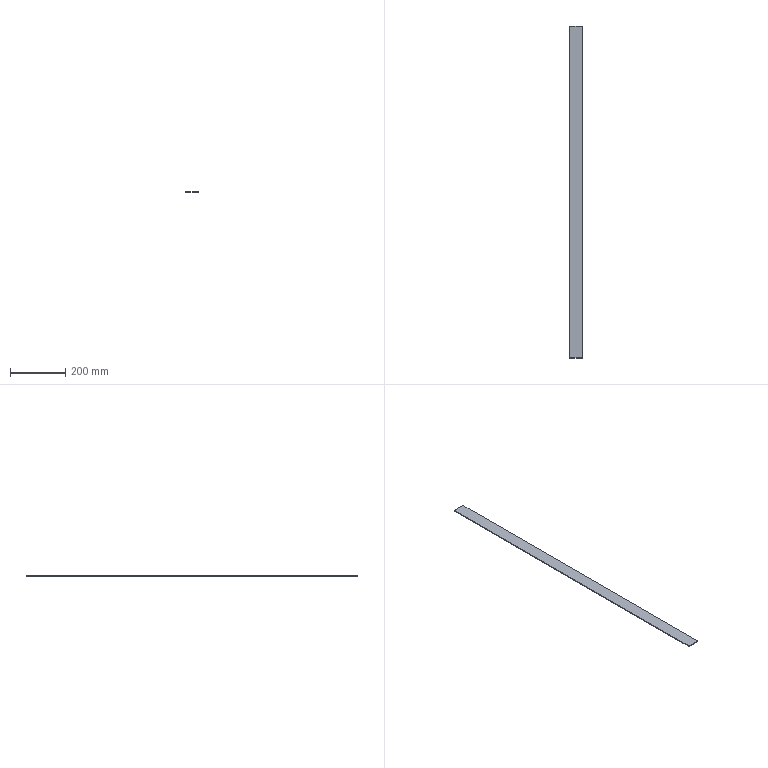Part | SolidWorks | features BaseBody 1 | 1 solid | 6 faces | box 44.635 x 1200 x 3 mm | volume 160685 mm3 | plane 6
STEP:
#1=CARTESIAN_POINT('',(171.506,600.,-1.5));
#2=VERTEX_POINT('',#1);
#3=CARTESIAN_POINT('',(171.506,-600.,-1.5));
#4=VERTEX_POINT('',#3);
#5=CARTESIAN_POINT('',(171.506,0.,-1.5));
#6=DIRECTION('',(0.,-1.,0.));
#7=VECTOR('',#6,1000.);
#8=LINE('',#5,#7);
#9=EDGE_CURVE('',#2,#4,#8,.T.);
#10=ORIENTED_EDGE('',*,*,#9,.T.);
#11=CARTESIAN_POINT('',(126.872,-600.,-1.5));
#12=VERTEX_POINT('',#11);
#13=CARTESIAN_POINT('',(149.189,-600.,-1.5));
#14=DIRECTION('',(-1.,0.,0.));
#15=VECTOR('',#14,1000.);
#16=LINE('',#13,#15);
#17=EDGE_CURVE('',#4,#12,#16,.T.);
#18=ORIENTED_EDGE('',*,*,#17,.T.);
#19=CARTESIAN_POINT('',(126.872,600.,-1.5));
#20=VERTEX_POINT('',#19);
#21=CARTESIAN_POINT('',(126.872,0.,-1.5));
#22=DIRECTION('',(0.,1.,0.));
#23=VECTOR('',#22,1000.);
#24=LINE('',#21,#23);
#25=EDGE_CURVE('',#12,#20,#24,.T.);
#26=ORIENTED_EDGE('',*,*,#25,.T.);
#27=CARTESIAN_POINT('',(149.189,600.,-1.5));
#28=DIRECTION('',(1.,0.,0.));
#29=VECTOR('',#28,1000.);
#30=LINE('',#27,#29);
#31=EDGE_CURVE('',#20,#2,#30,.T.);
#32=ORIENTED_EDGE('',*,*,#31,.T.);
#33=EDGE_LOOP('',(#10,#18,#26,#32));
#34=FACE_OUTER_BOUND('',#33,.T.);
#35=CARTESIAN_POINT('',(149.189,0.,-1.5));
#36=DIRECTION('',(0.,0.,-1.));
#37=DIRECTION('',(-1.,0.,0.));
#38=AXIS2_PLACEMENT_3D('',#35,#36,#37);
#39=PLANE('',#38);
#40=ADVANCED_FACE('',(#34),#39,.T.);
#41=CARTESIAN_POINT('',(126.872,-600.,1.5));
#42=VERTEX_POINT('',#41);
#43=CARTESIAN_POINT('',(126.872,-600.,0.));
#44=DIRECTION('',(0.,0.,-1.));
#45=VECTOR('',#44,1000.);
#46=LINE('',#43,#45);
#47=EDGE_CURVE('',#42,#12,#46,.T.);
#48=ORIENTED_EDGE('',*,*,#47,.T.);
#49=ORIENTED_EDGE('',*,*,#17,.F.);
#50=CARTESIAN_POINT('',(171.506,-600.,1.5));
#51=VERTEX_POINT('',#50);
#52=CARTESIAN_POINT('',(171.506,-600.,0.));
#53=DIRECTION('',(0.,0.,1.));
#54=VECTOR('',#53,1000.);
#55=LINE('',#52,#54);
#56=EDGE_CURVE('',#4,#51,#55,.T.);
#57=ORIENTED_EDGE('',*,*,#56,.T.);
#58=CARTESIAN_POINT('',(126.872,-600.,1.5));
#59=DIRECTION('',(-1.,0.,0.));
#60=VECTOR('',#59,1000.);
#61=LINE('',#58,#60);
#62=EDGE_CURVE('',#51,#42,#61,.T.);
#63=ORIENTED_EDGE('',*,*,#62,.T.);
#64=EDGE_LOOP('',(#48,#49,#57,#63));
#65=FACE_OUTER_BOUND('',#64,.T.);
#66=CARTESIAN_POINT('',(126.872,-600.,0.));
#67=DIRECTION('',(0.,-1.,0.));
#68=DIRECTION('',(1.,0.,0.));
#69=AXIS2_PLACEMENT_3D('',#66,#67,#68);
#70=PLANE('',#69);
#71=ADVANCED_FACE('',(#65),#70,.T.);
#72=ORIENTED_EDGE('',*,*,#56,.F.);
#73=ORIENTED_EDGE('',*,*,#9,.F.);
#74=CARTESIAN_POINT('',(171.506,600.,1.5));
#75=VERTEX_POINT('',#74);
#76=CARTESIAN_POINT('',(171.506,600.,0.));
#77=DIRECTION('',(0.,0.,1.));
#78=VECTOR('',#77,1000.);
#79=LINE('',#76,#78);
#80=EDGE_CURVE('',#2,#75,#79,.T.);
#81=ORIENTED_EDGE('',*,*,#80,.T.);
#82=CARTESIAN_POINT('',(171.506,-600.,1.5));
#83=DIRECTION('',(0.,-1.,0.));
#84=VECTOR('',#83,1000.);
#85=LINE('',#82,#84);
#86=EDGE_CURVE('',#75,#51,#85,.T.);
#87=ORIENTED_EDGE('',*,*,#86,.T.);
#88=EDGE_LOOP('',(#72,#73,#81,#87));
#89=FACE_OUTER_BOUND('',#88,.T.);
#90=CARTESIAN_POINT('',(171.506,-600.,0.));
#91=DIRECTION('',(1.,0.,0.));
#92=DIRECTION('',(0.,0.,-1.));
#93=AXIS2_PLACEMENT_3D('',#90,#91,#92);
#94=PLANE('',#93);
#95=ADVANCED_FACE('',(#89),#94,.T.);
#96=ORIENTED_EDGE('',*,*,#80,.F.);
#97=ORIENTED_EDGE('',*,*,#31,.F.);
#98=CARTESIAN_POINT('',(126.872,600.,1.5));
#99=VERTEX_POINT('',#98);
#100=CARTESIAN_POINT('',(126.872,600.,0.));
#101=DIRECTION('',(0.,0.,1.));
#102=VECTOR('',#101,1000.);
#103=LINE('',#100,#102);
#104=EDGE_CURVE('',#20,#99,#103,.T.);
#105=ORIENTED_EDGE('',*,*,#104,.T.);
#106=CARTESIAN_POINT('',(171.506,600.,1.5));
#107=DIRECTION('',(1.,0.,0.));
#108=VECTOR('',#107,1000.);
#109=LINE('',#106,#108);
#110=EDGE_CURVE('',#99,#75,#109,.T.);
#111=ORIENTED_EDGE('',*,*,#110,.T.);
#112=EDGE_LOOP('',(#96,#97,#105,#111));
#113=FACE_OUTER_BOUND('',#112,.T.);
#114=CARTESIAN_POINT('',(171.506,600.,0.));
#115=DIRECTION('',(0.,1.,0.));
#116=DIRECTION('',(-1.,0.,0.));
#117=AXIS2_PLACEMENT_3D('',#114,#115,#116);
#118=PLANE('',#117);
#119=ADVANCED_FACE('',(#113),#118,.T.);
#120=ORIENTED_EDGE('',*,*,#104,.F.);
#121=ORIENTED_EDGE('',*,*,#25,.F.);
#122=ORIENTED_EDGE('',*,*,#47,.F.);
#123=CARTESIAN_POINT('',(126.872,600.,1.5));
#124=DIRECTION('',(0.,1.,0.));
#125=VECTOR('',#124,1000.);
#126=LINE('',#123,#125);
#127=EDGE_CURVE('',#42,#99,#126,.T.);
#128=ORIENTED_EDGE('',*,*,#127,.T.);
#129=EDGE_LOOP('',(#120,#121,#122,#128));
#130=FACE_OUTER_BOUND('',#129,.T.);
#131=CARTESIAN_POINT('',(126.872,600.,0.));
#132=DIRECTION('',(-1.,0.,0.));
#133=DIRECTION('',(0.,0.,1.));
#134=AXIS2_PLACEMENT_3D('',#131,#132,#133);
#135=PLANE('',#134);
#136=ADVANCED_FACE('',(#130),#135,.T.);
#137=ORIENTED_EDGE('',*,*,#86,.F.);
#138=ORIENTED_EDGE('',*,*,#110,.F.);
#139=ORIENTED_EDGE('',*,*,#127,.F.);
#140=ORIENTED_EDGE('',*,*,#62,.F.);
#141=EDGE_LOOP('',(#137,#138,#139,#140));
#142=FACE_OUTER_BOUND('',#141,.T.);
#143=CARTESIAN_POINT('',(149.189,0.,1.5));
#144=DIRECTION('',(0.,0.,1.));
#145=DIRECTION('',(1.,0.,0.));
#146=AXIS2_PLACEMENT_3D('',#143,#144,#145);
#147=PLANE('',#146);
#148=ADVANCED_FACE('',(#142),#147,.T.);
#149=CLOSED_SHELL('',(#40,#71,#95,#119,#136,#148));
#150=MANIFOLD_SOLID_BREP('',#149);
#151=CARTESIAN_POINT('',(0.,0.,0.));
#152=DIRECTION('',(0.,0.,1.));
#153=DIRECTION('',(1.,0.,0.));
#154=AXIS2_PLACEMENT_3D('',#151,#152,#153);
#155=(LENGTH_UNIT()NAMED_UNIT(*)SI_UNIT(.MILLI.,.METRE.));
#156=UNCERTAINTY_MEASURE_WITH_UNIT(LENGTH_MEASURE(0.00001),#155,'','');
#157=(NAMED_UNIT(*)PLANE_ANGLE_UNIT()SI_UNIT($,.RADIAN.));
#158=(NAMED_UNIT(*)SI_UNIT($,.STERADIAN.)SOLID_ANGLE_UNIT());
#159=(GEOMETRIC_REPRESENTATION_CONTEXT(3)GLOBAL_UNCERTAINTY_ASSIGNED_CONTEXT((#156))GLOBAL_UNIT_ASSIGNED_CONTEXT((#155,#157,#158))REPRESENTATION_CONTEXT('',''));
#160=ADVANCED_BREP_SHAPE_REPRESENTATION('',(#150,#154),#159);